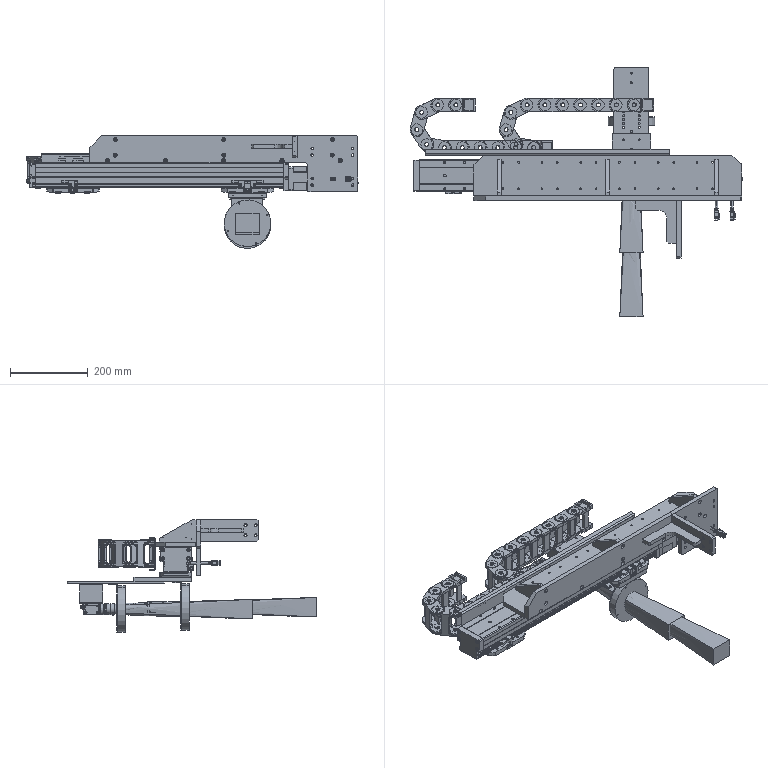Part | SolidWorks | features ReferencePattern 2, LocalLPattern 1 | 67 solids | 10646 faces | volume 8582117 mm3 | plane 5024 | cylinder 4445 | spline 580 | cone 577 | torus 20 | commonest cylinder face diameters 2 x931 4.24 x240 10 x223 18.2 x172 32.34 x166 13.7 x160